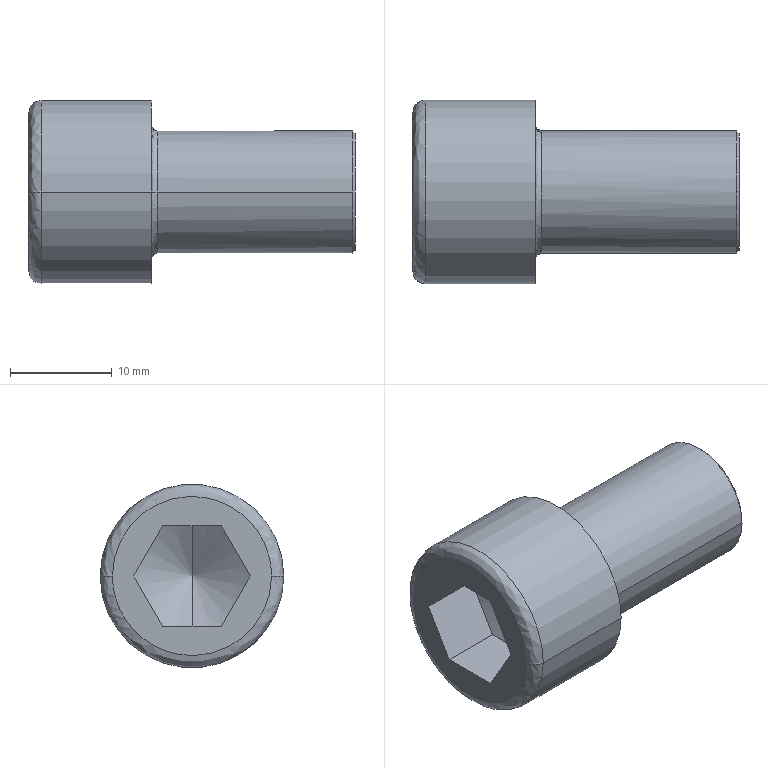Part | SolidWorks | features BaseBody 1 | 1 solid | 27 faces | box 32 x 18 x 18 mm | volume 4679 mm3 | plane 15 | spline 4 | cylinder 4 | cone 4 | commonest cylinder face diameters 12 x2 18 x2
STEP:
#1=CARTESIAN_POINT('',(0.6,6.,0.));
#2=VERTEX_POINT('',#1);
#3=CARTESIAN_POINT('',(0.6,-6.,0.));
#4=VERTEX_POINT('',#3);
#5=CARTESIAN_POINT('',(0.6,0.,0.));
#6=DIRECTION('',(1.,0.,0.));
#7=DIRECTION('',(0.,-1.,0.));
#8=AXIS2_PLACEMENT_3D('',#5,#6,#7);
#9=CIRCLE('',#8,6.);
#10=EDGE_CURVE('',#2,#4,#9,.T.);
#11=ORIENTED_EDGE('',*,*,#10,.F.);
#12=CARTESIAN_POINT('',(0.,6.6,0.));
#13=VERTEX_POINT('',#12);
#14=CARTESIAN_POINT('',(0.6,6.6,0.));
#15=DIRECTION('',(0.,0.,-1.));
#16=DIRECTION('',(0.,1.,0.));
#17=AXIS2_PLACEMENT_3D('',#14,#15,#16);
#18=CIRCLE('',#17,0.6);
#19=EDGE_CURVE('',#2,#13,#18,.T.);
#20=ORIENTED_EDGE('',*,*,#19,.T.);
#21=CARTESIAN_POINT('',(0.,-6.6,0.));
#22=VERTEX_POINT('',#21);
#23=CARTESIAN_POINT('',(0.,-6.6,0.));
#24=CARTESIAN_POINT('',(0.,-6.6,0.2019));
#25=CARTESIAN_POINT('',(0.,-6.586,0.5035));
#26=CARTESIAN_POINT('',(0.,-6.546,0.853));
#27=CARTESIAN_POINT('',(0.,-6.52,1.027));
#28=CARTESIAN_POINT('',(0.,-6.507,1.102));
#29=CARTESIAN_POINT('',(0.,-6.499,1.151));
#30=CARTESIAN_POINT('',(0.,-6.495,1.175));
#31=CARTESIAN_POINT('',(0.,-6.451,1.412));
#32=CARTESIAN_POINT('',(0.,-6.377,1.723));
#33=CARTESIAN_POINT('',(0.,-6.266,2.079));
#34=CARTESIAN_POINT('',(0.,-6.203,2.255));
#35=CARTESIAN_POINT('',(0.,-6.175,2.33));
#36=CARTESIAN_POINT('',(0.,-6.156,2.38));
#37=CARTESIAN_POINT('',(0.,-6.147,2.403));
#38=CARTESIAN_POINT('',(0.,-6.054,2.637));
#39=CARTESIAN_POINT('',(0.,-5.916,2.94));
#40=CARTESIAN_POINT('',(0.,-5.729,3.281));
#41=CARTESIAN_POINT('',(0.,-5.643,3.423));
#42=CARTESIAN_POINT('',(0.,-5.585,3.518));
#43=CARTESIAN_POINT('',(0.,-5.555,3.564));
#44=CARTESIAN_POINT('',(0.,-5.275,3.993));
#45=CARTESIAN_POINT('',(0.,-4.989,4.344));
#46=CARTESIAN_POINT('',(0.,-4.506,4.828));
#47=CARTESIAN_POINT('',(0.,-4.253,5.056));
#48=CARTESIAN_POINT('',(0.,-3.984,5.264));
#49=CARTESIAN_POINT('',(0.,-3.8,5.397));
#50=CARTESIAN_POINT('',(0.,-3.705,5.463));
#51=CARTESIAN_POINT('',(0.,-3.425,5.646));
#52=CARTESIAN_POINT('',(0.,-3.137,5.814));
#53=CARTESIAN_POINT('',(0.,-2.788,5.984));
#54=CARTESIAN_POINT('',(0.,-2.635,6.051));
#55=CARTESIAN_POINT('',(0.,-2.533,6.095));
#56=CARTESIAN_POINT('',(0.,-2.479,6.117));
#57=CARTESIAN_POINT('',(0.,-2.23,6.215));
#58=CARTESIAN_POINT('',(0.,-1.927,6.319));
#59=CARTESIAN_POINT('',(0.,-1.567,6.413));
#60=CARTESIAN_POINT('',(0.,-1.384,6.454));
#61=CARTESIAN_POINT('',(0.,-1.306,6.47));
#62=CARTESIAN_POINT('',(0.,-1.253,6.48));
#63=CARTESIAN_POINT('',(0.,-1.226,6.485));
#64=CARTESIAN_POINT('',(0.,-0.8037,6.563));
#65=CARTESIAN_POINT('',(0.,-0.404,6.6));
#66=CARTESIAN_POINT('',(0.,0.202,6.6));
#67=CARTESIAN_POINT('',(0.,0.5037,6.586));
#68=CARTESIAN_POINT('',(0.,0.8531,6.546));
#69=CARTESIAN_POINT('',(0.,1.027,6.52));
#70=CARTESIAN_POINT('',(0.,1.102,6.507));
#71=CARTESIAN_POINT('',(0.,1.151,6.499));
#72=CARTESIAN_POINT('',(0.,1.175,6.495));
#73=CARTESIAN_POINT('',(0.,1.412,6.451));
#74=CARTESIAN_POINT('',(0.,1.723,6.377));
#75=CARTESIAN_POINT('',(0.,2.079,6.266));
#76=CARTESIAN_POINT('',(0.,2.255,6.203));
#77=CARTESIAN_POINT('',(0.,2.33,6.175));
#78=CARTESIAN_POINT('',(0.,2.38,6.156));
#79=CARTESIAN_POINT('',(0.,2.403,6.147));
#80=CARTESIAN_POINT('',(0.,2.637,6.054));
#81=CARTESIAN_POINT('',(0.,2.94,5.916));
#82=CARTESIAN_POINT('',(0.,3.281,5.729));
#83=CARTESIAN_POINT('',(0.,3.423,5.643));
#84=CARTESIAN_POINT('',(0.,3.518,5.585));
#85=CARTESIAN_POINT('',(0.,3.564,5.555));
#86=CARTESIAN_POINT('',(0.,3.993,5.275));
#87=CARTESIAN_POINT('',(0.,4.344,4.989));
#88=CARTESIAN_POINT('',(0.,4.828,4.506));
#89=CARTESIAN_POINT('',(0.,5.056,4.253));
#90=CARTESIAN_POINT('',(0.,5.264,3.984));
#91=CARTESIAN_POINT('',(0.,5.397,3.8));
#92=CARTESIAN_POINT('',(0.,5.463,3.705));
#93=CARTESIAN_POINT('',(0.,5.646,3.425));
#94=CARTESIAN_POINT('',(0.,5.814,3.137));
#95=CARTESIAN_POINT('',(0.,5.984,2.788));
#96=CARTESIAN_POINT('',(0.,6.051,2.635));
#97=CARTESIAN_POINT('',(0.,6.095,2.533));
#98=CARTESIAN_POINT('',(0.,6.117,2.479));
#99=CARTESIAN_POINT('',(0.,6.215,2.23));
#100=CARTESIAN_POINT('',(0.,6.319,1.927));
#101=CARTESIAN_POINT('',(0.,6.413,1.567));
#102=CARTESIAN_POINT('',(0.,6.454,1.384));
#103=CARTESIAN_POINT('',(0.,6.47,1.306));
#104=CARTESIAN_POINT('',(0.,6.48,1.253));
#105=CARTESIAN_POINT('',(0.,6.485,1.226));
#106=CARTESIAN_POINT('',(0.,6.563,0.8038));
#107=CARTESIAN_POINT('',(0.,6.6,0.4035));
#108=CARTESIAN_POINT('',(0.,6.6,0.));
#109=B_SPLINE_CURVE_WITH_KNOTS('',3,(#23,#24,#25,#26,#27,#28,#29,#30,#31,#32,#33,#34,#35,#36,#37,#38,#39,#40,#41,#42,#43,#44,#45,#46,#47,#48,#49,#50,#51,#52,#53,#54,#55,#56,#57,#58,#59,#60,#61,#62,#63,#64,#65,#66,#67,#68,#69,#70,#71,#72,#73,#74,#75,#76,#77,#78,#79,#80,#81,#82,#83,#84,#85,#86,#87,#88,#89,#90,#91,#92,#93,#94,#95,#96,#97,#98,#99,#100,#101,#102,#103,#104,#105,#106,#107,#108),.UNSPECIFIED.,.F.,.F.,(4,1,1,1,2,2,1,1,1,2,2,1,1,2,2,2,1,2,2,1,1,2,2,1,1,1,2,2,2,1,1,1,2,2,1,1,1,2,2,1,1,2,2,2,1,2,2,1,1,2,2,1,1,1,2,2,4),(0.,0.03125,0.04688,0.05469,0.05859,0.0625,0.09375,0.1094,0.1172,0.1211,0.125,0.1563,0.1719,0.1797,0.1875,0.25,0.2813,0.2969,0.3125,0.3438,0.3594,0.3672,0.375,0.4063,0.4219,0.4297,0.4336,0.4375,0.5,0.5313,0.5469,0.5547,0.5586,0.5625,0.5938,0.6094,0.6172,0.6211,0.625,0.6563,0.6719,0.6797,0.6875,0.75,0.7813,0.7969,0.8125,0.8438,0.8594,0.8672,0.875,0.9063,0.9219,0.9297,0.9336,0.9375,1.),.UNSPECIFIED.);
#110=EDGE_CURVE('',#22,#13,#109,.T.);
#111=ORIENTED_EDGE('',*,*,#110,.F.);
#112=CARTESIAN_POINT('',(0.6,-6.6,0.));
#113=DIRECTION('',(0.,0.,1.));
#114=DIRECTION('',(0.,-1.,0.));
#115=AXIS2_PLACEMENT_3D('',#112,#113,#114);
#116=CIRCLE('',#115,0.6);
#117=EDGE_CURVE('',#4,#22,#116,.T.);
#118=ORIENTED_EDGE('',*,*,#117,.F.);
#119=EDGE_LOOP('',(#11,#20,#111,#118));
#120=FACE_OUTER_BOUND('',#119,.T.);
#121=CARTESIAN_POINT('',(0.6,-6.,0.));
#122=CARTESIAN_POINT('',(0.6,-6.,12.));
#123=CARTESIAN_POINT('',(0.6,6.,12.));
#124=CARTESIAN_POINT('',(0.6,6.,0.));
#125=CARTESIAN_POINT('',(0.2485,-6.,0.));
#126=CARTESIAN_POINT('',(0.2485,-6.,12.));
#127=CARTESIAN_POINT('',(0.2485,6.,12.));
#128=CARTESIAN_POINT('',(0.2485,6.,0.));
#129=CARTESIAN_POINT('',(0.,-6.249,0.));
#130=CARTESIAN_POINT('',(0.,-6.249,12.497));
#131=CARTESIAN_POINT('',(0.,6.249,12.497));
#132=CARTESIAN_POINT('',(0.,6.249,0.));
#133=CARTESIAN_POINT('',(0.,-6.6,0.));
#134=CARTESIAN_POINT('',(0.,-6.6,13.2));
#135=CARTESIAN_POINT('',(0.,6.6,13.2));
#136=CARTESIAN_POINT('',(0.,6.6,0.));
#137=(BOUNDED_SURFACE()B_SPLINE_SURFACE(3,3,((#121,#122,#123,#124),(#125,#126,#127,#128),(#129,#130,#131,#132),(#133,#134,#135,#136)),.UNSPECIFIED.,.F.,.F.,.T.)B_SPLINE_SURFACE_WITH_KNOTS((4,4),(4,4),(0.,1.),(0.,1.),.UNSPECIFIED.)GEOMETRIC_REPRESENTATION_ITEM()RATIONAL_B_SPLINE_SURFACE(((1.,0.3333,0.3333,1.),(0.8047,0.2682,0.2682,0.8047),(0.8047,0.2682,0.2682,0.8047),(1.,0.3333,0.3333,1.)))REPRESENTATION_ITEM('')SURFACE());
#138=ADVANCED_FACE('',(#120),#137,.F.);
#139=CARTESIAN_POINT('',(-10.8,-9.,0.));
#140=VERTEX_POINT('',#139);
#141=CARTESIAN_POINT('',(-10.8,9.,0.));
#142=VERTEX_POINT('',#141);
#143=CARTESIAN_POINT('',(-10.8,0.,0.));
#144=DIRECTION('',(1.,0.,0.));
#145=DIRECTION('',(0.,-1.,0.));
#146=AXIS2_PLACEMENT_3D('',#143,#144,#145);
#147=CIRCLE('',#146,9.);
#148=EDGE_CURVE('',#140,#142,#147,.T.);
#149=ORIENTED_EDGE('',*,*,#148,.F.);
#150=CARTESIAN_POINT('',(-12.,-7.8,0.));
#151=VERTEX_POINT('',#150);
#152=CARTESIAN_POINT('',(-10.8,-7.8,0.));
#153=DIRECTION('',(0.,0.,-1.));
#154=DIRECTION('',(0.,-1.,0.));
#155=AXIS2_PLACEMENT_3D('',#152,#153,#154);
#156=CIRCLE('',#155,1.2);
#157=EDGE_CURVE('',#140,#151,#156,.T.);
#158=ORIENTED_EDGE('',*,*,#157,.T.);
#159=CARTESIAN_POINT('',(-12.,7.8,0.));
#160=VERTEX_POINT('',#159);
#161=CARTESIAN_POINT('',(-12.,-7.8,0.));
#162=CARTESIAN_POINT('',(-12.,-7.8,-15.6));
#163=CARTESIAN_POINT('',(-12.,7.8,-15.6));
#164=CARTESIAN_POINT('',(-12.,7.8,0.));
#165=(BOUNDED_CURVE()B_SPLINE_CURVE(3,(#161,#162,#163,#164),.UNSPECIFIED.,.F.,.F.)B_SPLINE_CURVE_WITH_KNOTS((4,4),(0.,1.),.UNSPECIFIED.)CURVE()GEOMETRIC_REPRESENTATION_ITEM()RATIONAL_B_SPLINE_CURVE((1.,0.3333,0.3333,1.))REPRESENTATION_ITEM(''));
#166=EDGE_CURVE('',#151,#160,#165,.T.);
#167=ORIENTED_EDGE('',*,*,#166,.T.);
#168=CARTESIAN_POINT('',(-10.8,7.8,0.));
#169=DIRECTION('',(0.,0.,1.));
#170=DIRECTION('',(0.,1.,0.));
#171=AXIS2_PLACEMENT_3D('',#168,#169,#170);
#172=CIRCLE('',#171,1.2);
#173=EDGE_CURVE('',#142,#160,#172,.T.);
#174=ORIENTED_EDGE('',*,*,#173,.F.);
#175=EDGE_LOOP('',(#149,#158,#167,#174));
#176=FACE_OUTER_BOUND('',#175,.T.);
#177=CARTESIAN_POINT('',(-10.8,-9.,0.));
#178=CARTESIAN_POINT('',(-10.8,-9.,-18.));
#179=CARTESIAN_POINT('',(-10.8,9.,-18.));
#180=CARTESIAN_POINT('',(-10.8,9.,0.));
#181=CARTESIAN_POINT('',(-11.503,-9.,0.));
#182=CARTESIAN_POINT('',(-11.503,-9.,-18.));
#183=CARTESIAN_POINT('',(-11.503,9.,-18.));
#184=CARTESIAN_POINT('',(-11.503,9.,0.));
#185=CARTESIAN_POINT('',(-12.,-8.503,0.));
#186=CARTESIAN_POINT('',(-12.,-8.503,-17.006));
#187=CARTESIAN_POINT('',(-12.,8.503,-17.006));
#188=CARTESIAN_POINT('',(-12.,8.503,0.));
#189=CARTESIAN_POINT('',(-12.,-7.8,0.));
#190=CARTESIAN_POINT('',(-12.,-7.8,-15.6));
#191=CARTESIAN_POINT('',(-12.,7.8,-15.6));
#192=CARTESIAN_POINT('',(-12.,7.8,0.));
#193=(BOUNDED_SURFACE()B_SPLINE_SURFACE(3,3,((#177,#178,#179,#180),(#181,#182,#183,#184),(#185,#186,#187,#188),(#189,#190,#191,#192)),.UNSPECIFIED.,.F.,.F.,.T.)B_SPLINE_SURFACE_WITH_KNOTS((4,4),(4,4),(0.,1.),(0.,1.),.UNSPECIFIED.)GEOMETRIC_REPRESENTATION_ITEM()RATIONAL_B_SPLINE_SURFACE(((1.,0.3333,0.3333,1.),(0.8047,0.2682,0.2682,0.8047),(0.8047,0.2682,0.2682,0.8047),(1.,0.3333,0.3333,1.)))REPRESENTATION_ITEM('')SURFACE());
#194=ADVANCED_FACE('',(#176),#193,.T.);
#195=CARTESIAN_POINT('',(19.76,0.,6.));
#196=VERTEX_POINT('',#195);
#197=CARTESIAN_POINT('',(19.76,6.,0.));
#198=VERTEX_POINT('',#197);
#199=CARTESIAN_POINT('',(19.76,0.,0.));
#200=DIRECTION('',(-1.,0.,0.));
#201=DIRECTION('',(0.,-1.,0.));
#202=AXIS2_PLACEMENT_3D('',#199,#200,#201);
#203=CIRCLE('',#202,6.);
#204=EDGE_CURVE('',#196,#198,#203,.T.);
#205=ORIENTED_EDGE('',*,*,#204,.T.);
#206=CARTESIAN_POINT('',(20.,6.,0.));
#207=DIRECTION('',(-1.,0.,0.));
#208=VECTOR('',#207,1000.);
#209=LINE('',#206,#208);
#210=EDGE_CURVE('',#198,#2,#209,.T.);
#211=ORIENTED_EDGE('',*,*,#210,.T.);
#212=ORIENTED_EDGE('',*,*,#10,.T.);
#213=CARTESIAN_POINT('',(19.76,-6.,0.));
#214=VERTEX_POINT('',#213);
#215=CARTESIAN_POINT('',(20.,-6.,0.));
#216=DIRECTION('',(-1.,0.,0.));
#217=VECTOR('',#216,1000.);
#218=LINE('',#215,#217);
#219=EDGE_CURVE('',#214,#4,#218,.T.);
#220=ORIENTED_EDGE('',*,*,#219,.F.);
#221=CARTESIAN_POINT('',(19.76,0.,0.));
#222=DIRECTION('',(-1.,0.,0.));
#223=DIRECTION('',(0.,-1.,0.));
#224=AXIS2_PLACEMENT_3D('',#221,#222,#223);
#225=CIRCLE('',#224,6.);
#226=EDGE_CURVE('',#214,#196,#225,.T.);
#227=ORIENTED_EDGE('',*,*,#226,.T.);
#228=EDGE_LOOP('',(#205,#211,#212,#220,#227));
#229=FACE_OUTER_BOUND('',#228,.T.);
#230=CARTESIAN_POINT('',(20.,0.,0.));
#231=DIRECTION('',(-1.,0.,0.));
#232=DIRECTION('',(0.,-1.,0.));
#233=AXIS2_PLACEMENT_3D('',#230,#231,#232);
#234=CYLINDRICAL_SURFACE('',#233,6.);
#235=ADVANCED_FACE('',(#229),#234,.T.);
#236=CARTESIAN_POINT('',(20.,0.,5.76));
#237=VERTEX_POINT('',#236);
#238=CARTESIAN_POINT('',(20.,0.,-5.76));
#239=VERTEX_POINT('',#238);
#240=CARTESIAN_POINT('',(20.,0.,0.));
#241=DIRECTION('',(-1.,0.,0.));
#242=DIRECTION('',(0.,0.,1.));
#243=AXIS2_PLACEMENT_3D('',#240,#241,#242);
#244=CIRCLE('',#243,5.76);
#245=EDGE_CURVE('',#237,#239,#244,.T.);
#246=ORIENTED_EDGE('',*,*,#245,.T.);
#247=CARTESIAN_POINT('',(19.76,0.,-6.));
#248=VERTEX_POINT('',#247);
#249=CARTESIAN_POINT('',(19.76,0.,-6.));
#250=DIRECTION('',(-0.7071,0.,-0.7071));
#251=VECTOR('',#250,1000.);
#252=LINE('',#249,#251);
#253=EDGE_CURVE('',#239,#248,#252,.T.);
#254=ORIENTED_EDGE('',*,*,#253,.T.);
#255=CARTESIAN_POINT('',(19.76,0.,0.));
#256=DIRECTION('',(-1.,0.,0.));
#257=DIRECTION('',(0.,-1.,0.));
#258=AXIS2_PLACEMENT_3D('',#255,#256,#257);
#259=CIRCLE('',#258,6.);
#260=EDGE_CURVE('',#198,#248,#259,.T.);
#261=ORIENTED_EDGE('',*,*,#260,.F.);
#262=ORIENTED_EDGE('',*,*,#204,.F.);
#263=CARTESIAN_POINT('',(19.76,0.,6.));
#264=DIRECTION('',(-0.7071,0.,0.7071));
#265=VECTOR('',#264,1000.);
#266=LINE('',#263,#265);
#267=EDGE_CURVE('',#237,#196,#266,.T.);
#268=ORIENTED_EDGE('',*,*,#267,.F.);
#269=EDGE_LOOP('',(#246,#254,#261,#262,#268));
#270=FACE_OUTER_BOUND('',#269,.T.);
#271=CARTESIAN_POINT('',(19.76,0.,0.));
#272=DIRECTION('',(-1.,0.,0.));
#273=DIRECTION('',(0.,0.,1.));
#274=AXIS2_PLACEMENT_3D('',#271,#272,#273);
#275=CONICAL_SURFACE('',#274,6.,0.7854);
#276=ADVANCED_FACE('',(#270),#275,.T.);
#277=CARTESIAN_POINT('',(0.,-9.,0.));
#278=VERTEX_POINT('',#277);
#279=CARTESIAN_POINT('',(0.,9.,0.));
#280=VERTEX_POINT('',#279);
#281=CARTESIAN_POINT('',(0.,0.,0.));
#282=DIRECTION('',(-1.,0.,0.));
#283=DIRECTION('',(0.,-1.,0.));
#284=AXIS2_PLACEMENT_3D('',#281,#282,#283);
#285=CIRCLE('',#284,9.);
#286=EDGE_CURVE('',#278,#280,#285,.T.);
#287=ORIENTED_EDGE('',*,*,#286,.T.);
#288=CARTESIAN_POINT('',(-2.701,9.,0.));
#289=DIRECTION('',(-1.,0.,0.));
#290=VECTOR('',#289,1000.);
#291=LINE('',#288,#290);
#292=EDGE_CURVE('',#280,#142,#291,.T.);
#293=ORIENTED_EDGE('',*,*,#292,.T.);
#294=CARTESIAN_POINT('',(-10.8,0.,0.));
#295=DIRECTION('',(1.,0.,0.));
#296=DIRECTION('',(0.,-1.,0.));
#297=AXIS2_PLACEMENT_3D('',#294,#295,#296);
#298=CIRCLE('',#297,9.);
#299=EDGE_CURVE('',#142,#140,#298,.T.);
#300=ORIENTED_EDGE('',*,*,#299,.T.);
#301=CARTESIAN_POINT('',(-2.701,-9.,0.));
#302=DIRECTION('',(-1.,0.,0.));
#303=VECTOR('',#302,1000.);
#304=LINE('',#301,#303);
#305=EDGE_CURVE('',#278,#140,#304,.T.);
#306=ORIENTED_EDGE('',*,*,#305,.F.);
#307=EDGE_LOOP('',(#287,#293,#300,#306));
#308=FACE_OUTER_BOUND('',#307,.T.);
#309=CARTESIAN_POINT('',(-2.701,0.,0.));
#310=DIRECTION('',(-1.,0.,0.));
#311=DIRECTION('',(0.,-1.,0.));
#312=AXIS2_PLACEMENT_3D('',#309,#310,#311);
#313=CYLINDRICAL_SURFACE('',#312,9.);
#314=ADVANCED_FACE('',(#308),#313,.T.);
#315=CARTESIAN_POINT('',(-2.701,0.,0.));
#316=VERTEX_POINT('',#315);
#317=CARTESIAN_POINT('',(-6.,0.,5.715));
#318=VERTEX_POINT('',#317);
#319=CARTESIAN_POINT('',(-6.,0.,5.715));
#320=DIRECTION('',(-0.5,0.,0.866));
#321=VECTOR('',#320,1000.);
#322=LINE('',#319,#321);
#323=EDGE_CURVE('',#316,#318,#322,.T.);
#324=ORIENTED_EDGE('',*,*,#323,.F.);
#325=CARTESIAN_POINT('',(-6.,0.,-5.714));
#326=VERTEX_POINT('',#325);
#327=CARTESIAN_POINT('',(-6.,0.,-5.715));
#328=DIRECTION('',(-0.5,0.,-0.866));
#329=VECTOR('',#328,1000.);
#330=LINE('',#327,#329);
#331=EDGE_CURVE('',#316,#326,#330,.T.);
#332=ORIENTED_EDGE('',*,*,#331,.T.);
#333=CARTESIAN_POINT('',(-6.,-2.857,-4.949));
#334=VERTEX_POINT('',#333);
#335=CARTESIAN_POINT('',(-6.,0.,0.));
#336=DIRECTION('',(-1.,0.,0.));
#337=DIRECTION('',(0.,0.,1.));
#338=AXIS2_PLACEMENT_3D('',#335,#336,#337);
#339=CIRCLE('',#338,5.715);
#340=EDGE_CURVE('',#326,#334,#339,.T.);
#341=ORIENTED_EDGE('',*,*,#340,.T.);
#342=CARTESIAN_POINT('',(-6.,-5.715,0.));
#343=VERTEX_POINT('',#342);
#344=CARTESIAN_POINT('',(-6.,0.,0.));
#345=DIRECTION('',(-1.,0.,0.));
#346=DIRECTION('',(0.,0.,1.));
#347=AXIS2_PLACEMENT_3D('',#344,#345,#346);
#348=CIRCLE('',#347,5.715);
#349=EDGE_CURVE('',#334,#343,#348,.T.);
#350=ORIENTED_EDGE('',*,*,#349,.T.);
#351=CARTESIAN_POINT('',(-6.,-2.857,4.949));
#352=VERTEX_POINT('',#351);
#353=CARTESIAN_POINT('',(-6.,0.,0.));
#354=DIRECTION('',(-1.,0.,0.));
#355=DIRECTION('',(0.,0.,1.));
#356=AXIS2_PLACEMENT_3D('',#353,#354,#355);
#357=CIRCLE('',#356,5.715);
#358=EDGE_CURVE('',#343,#352,#357,.T.);
#359=ORIENTED_EDGE('',*,*,#358,.T.);
#360=CARTESIAN_POINT('',(-6.,0.,0.));
#361=DIRECTION('',(-1.,0.,0.));
#362=DIRECTION('',(0.,0.,1.));
#363=AXIS2_PLACEMENT_3D('',#360,#361,#362);
#364=CIRCLE('',#363,5.715);
#365=EDGE_CURVE('',#352,#318,#364,.T.);
#366=ORIENTED_EDGE('',*,*,#365,.T.);
#367=EDGE_LOOP('',(#324,#332,#341,#350,#359,#366));
#368=FACE_OUTER_BOUND('',#367,.T.);
#369=CARTESIAN_POINT('',(-6.,0.,0.));
#370=DIRECTION('',(-1.,0.,0.));
#371=DIRECTION('',(0.,0.,1.));
#372=AXIS2_PLACEMENT_3D('',#369,#370,#371);
#373=CONICAL_SURFACE('',#372,5.715,1.047);
#374=ADVANCED_FACE('',(#368),#373,.F.);
#375=ORIENTED_EDGE('',*,*,#210,.F.);
#376=ORIENTED_EDGE('',*,*,#260,.T.);
#377=CARTESIAN_POINT('',(19.76,0.,0.));
#378=DIRECTION('',(-1.,0.,0.));
#379=DIRECTION('',(0.,-1.,0.));
#380=AXIS2_PLACEMENT_3D('',#377,#378,#379);
#381=CIRCLE('',#380,6.);
#382=EDGE_CURVE('',#248,#214,#381,.T.);
#383=ORIENTED_EDGE('',*,*,#382,.T.);
#384=ORIENTED_EDGE('',*,*,#219,.T.);
#385=CARTESIAN_POINT('',(0.6,0.,0.));
#386=DIRECTION('',(1.,0.,0.));
#387=DIRECTION('',(0.,-1.,0.));
#388=AXIS2_PLACEMENT_3D('',#385,#386,#387);
#389=CIRCLE('',#388,6.);
#390=EDGE_CURVE('',#4,#2,#389,.T.);
#391=ORIENTED_EDGE('',*,*,#390,.T.);
#392=EDGE_LOOP('',(#375,#376,#383,#384,#391));
#393=FACE_OUTER_BOUND('',#392,.T.);
#394=CARTESIAN_POINT('',(20.,0.,0.));
#395=DIRECTION('',(-1.,0.,0.));
#396=DIRECTION('',(0.,-1.,0.));
#397=AXIS2_PLACEMENT_3D('',#394,#395,#396);
#398=CYLINDRICAL_SURFACE('',#397,6.);
#399=ADVANCED_FACE('',(#393),#398,.T.);
#400=ORIENTED_EDGE('',*,*,#19,.F.);
#401=ORIENTED_EDGE('',*,*,#390,.F.);
#402=ORIENTED_EDGE('',*,*,#117,.T.);
#403=CARTESIAN_POINT('',(0.,6.6,0.));
#404=CARTESIAN_POINT('',(0.,6.6,-0.2019));
#405=CARTESIAN_POINT('',(0.,6.586,-0.5035));
#406=CARTESIAN_POINT('',(0.,6.546,-0.853));
#407=CARTESIAN_POINT('',(0.,6.52,-1.027));
#408=CARTESIAN_POINT('',(0.,6.507,-1.102));
#409=CARTESIAN_POINT('',(0.,6.499,-1.151));
#410=CARTESIAN_POINT('',(0.,6.495,-1.175));
#411=CARTESIAN_POINT('',(0.,6.451,-1.412));
#412=CARTESIAN_POINT('',(0.,6.377,-1.723));
#413=CARTESIAN_POINT('',(0.,6.266,-2.079));
#414=CARTESIAN_POINT('',(0.,6.203,-2.255));
#415=CARTESIAN_POINT('',(0.,6.175,-2.33));
#416=CARTESIAN_POINT('',(0.,6.156,-2.38));
#417=CARTESIAN_POINT('',(0.,6.147,-2.403));
#418=CARTESIAN_POINT('',(0.,6.054,-2.637));
#419=CARTESIAN_POINT('',(0.,5.916,-2.94));
#420=CARTESIAN_POINT('',(0.,5.729,-3.281));
#421=CARTESIAN_POINT('',(0.,5.643,-3.423));
#422=CARTESIAN_POINT('',(0.,5.585,-3.518));
#423=CARTESIAN_POINT('',(0.,5.555,-3.564));
#424=CARTESIAN_POINT('',(0.,5.275,-3.993));
#425=CARTESIAN_POINT('',(0.,4.989,-4.344));
#426=CARTESIAN_POINT('',(0.,4.506,-4.828));
#427=CARTESIAN_POINT('',(0.,4.253,-5.056));
#428=CARTESIAN_POINT('',(0.,3.984,-5.264));
#429=CARTESIAN_POINT('',(0.,3.8,-5.397));
#430=CARTESIAN_POINT('',(0.,3.705,-5.463));
#431=CARTESIAN_POINT('',(0.,3.425,-5.646));
#432=CARTESIAN_POINT('',(0.,3.137,-5.814));
#433=CARTESIAN_POINT('',(0.,2.788,-5.984));
#434=CARTESIAN_POINT('',(0.,2.635,-6.051));
#435=CARTESIAN_POINT('',(0.,2.533,-6.095));
#436=CARTESIAN_POINT('',(0.,2.479,-6.117));
#437=CARTESIAN_POINT('',(0.,2.23,-6.215));
#438=CARTESIAN_POINT('',(0.,1.927,-6.319));
#439=CARTESIAN_POINT('',(0.,1.567,-6.413));
#440=CARTESIAN_POINT('',(0.,1.384,-6.454));
#441=CARTESIAN_POINT('',(0.,1.306,-6.47));
#442=CARTESIAN_POINT('',(0.,1.253,-6.48));
#443=CARTESIAN_POINT('',(0.,1.226,-6.485));
#444=CARTESIAN_POINT('',(0.,0.8037,-6.563));
#445=CARTESIAN_POINT('',(0.,0.404,-6.6));
#446=CARTESIAN_POINT('',(0.,-0.202,-6.6));
#447=CARTESIAN_POINT('',(0.,-0.5037,-6.586));
#448=CARTESIAN_POINT('',(0.,-0.8531,-6.546));
#449=CARTESIAN_POINT('',(0.,-1.027,-6.52));
#450=CARTESIAN_POINT('',(0.,-1.102,-6.507));
#451=CARTESIAN_POINT('',(0.,-1.151,-6.499));
#452=CARTESIAN_POINT('',(0.,-1.175,-6.495));
#453=CARTESIAN_POINT('',(0.,-1.412,-6.451));
#454=CARTESIAN_POINT('',(0.,-1.723,-6.377));
#455=CARTESIAN_POINT('',(0.,-2.079,-6.266));
#456=CARTESIAN_POINT('',(0.,-2.255,-6.203));
#457=CARTESIAN_POINT('',(0.,-2.33,-6.175));
#458=CARTESIAN_POINT('',(0.,-2.38,-6.156));
#459=CARTESIAN_POINT('',(0.,-2.403,-6.147));
#460=CARTESIAN_POINT('',(0.,-2.637,-6.054));
#461=CARTESIAN_POINT('',(0.,-2.94,-5.916));
#462=CARTESIAN_POINT('',(0.,-3.281,-5.729));
#463=CARTESIAN_POINT('',(0.,-3.423,-5.643));
#464=CARTESIAN_POINT('',(0.,-3.518,-5.585));
#465=CARTESIAN_POINT('',(0.,-3.564,-5.555));
#466=CARTESIAN_POINT('',(0.,-3.993,-5.275));
#467=CARTESIAN_POINT('',(0.,-4.344,-4.989));
#468=CARTESIAN_POINT('',(0.,-4.828,-4.506));
#469=CARTESIAN_POINT('',(0.,-5.056,-4.253));
#470=CARTESIAN_POINT('',(0.,-5.264,-3.984));
#471=CARTESIAN_POINT('',(0.,-5.397,-3.8));
#472=CARTESIAN_POINT('',(0.,-5.463,-3.705));
#473=CARTESIAN_POINT('',(0.,-5.646,-3.425));
#474=CARTESIAN_POINT('',(0.,-5.814,-3.137));
#475=CARTESIAN_POINT('',(0.,-5.984,-2.788));
#476=CARTESIAN_POINT('',(0.,-6.051,-2.635));
#477=CARTESIAN_POINT('',(0.,-6.095,-2.533));
#478=CARTESIAN_POINT('',(0.,-6.117,-2.479));
#479=CARTESIAN_POINT('',(0.,-6.215,-2.23));
#480=CARTESIAN_POINT('',(0.,-6.319,-1.927));
#481=CARTESIAN_POINT('',(0.,-6.413,-1.567));
#482=CARTESIAN_POINT('',(0.,-6.454,-1.384));
#483=CARTESIAN_POINT('',(0.,-6.47,-1.306));
#484=CARTESIAN_POINT('',(0.,-6.48,-1.253));
#485=CARTESIAN_POINT('',(0.,-6.485,-1.226));
#486=CARTESIAN_POINT('',(0.,-6.563,-0.8038));
#487=CARTESIAN_POINT('',(0.,-6.6,-0.4035));
#488=CARTESIAN_POINT('',(0.,-6.6,0.));
#489=B_SPLINE_CURVE_WITH_KNOTS('',3,(#403,#404,#405,#406,#407,#408,#409,#410,#411,#412,#413,#414,#415,#416,#417,#418,#419,#420,#421,#422,#423,#424,#425,#426,#427,#428,#429,#430,#431,#432,#433,#434,#435,#436,#437,#438,#439,#440,#441,#442,#443,#444,#445,#446,#447,#448,#449,#450,#451,#452,#453,#454,#455,#456,#457,#458,#459,#460,#461,#462,#463,#464,#465,#466,#467,#468,#469,#470,#471,#472,#473,#474,#475,#476,#477,#478,#479,#480,#481,#482,#483,#484,#485,#486,#487,#488),.UNSPECIFIED.,.F.,.F.,(4,1,1,1,2,2,1,1,1,2,2,1,1,2,2,2,1,2,2,1,1,2,2,1,1,1,2,2,2,1,1,1,2,2,1,1,1,2,2,1,1,2,2,2,1,2,2,1,1,2,2,1,1,1,2,2,4),(0.,0.03125,0.04688,0.05469,0.05859,0.0625,0.09375,0.1094,0.1172,0.1211,0.125,0.1563,0.1719,0.1797,0.1875,0.25,0.2813,0.2969,0.3125,0.3437,0.3594,0.3672,0.375,0.4062,0.4219,0.4297,0.4336,0.4375,0.5,0.5312,0.5469,0.5547,0.5586,0.5625,0.5937,0.6094,0.6172,0.6211,0.625,0.6562,0.6719,0.6797,0.6875,0.75,0.7812,0.7969,0.8125,0.8437,0.8594,0.8672,0.875,0.9062,0.9219,0.9297,0.9336,0.9375,1.),.UNSPECIFIED.);
#490=EDGE_CURVE('',#13,#22,#489,.T.);
#491=ORIENTED_EDGE('',*,*,#490,.F.);
#492=EDGE_LOOP('',(#400,#401,#402,#491));
#493=FACE_OUTER_BOUND('',#492,.T.);
#494=CARTESIAN_POINT('',(0.6,6.,0.));
#495=CARTESIAN_POINT('',(0.6,6.,-12.));
#496=CARTESIAN_POINT('',(0.6,-6.,-12.));
#497=CARTESIAN_POINT('',(0.6,-6.,0.));
#498=CARTESIAN_POINT('',(0.2485,6.,0.));
#499=CARTESIAN_POINT('',(0.2485,6.,-12.));
#500=CARTESIAN_POINT('',(0.2485,-6.,-12.));
#501=CARTESIAN_POINT('',(0.2485,-6.,0.));
#502=CARTESIAN_POINT('',(0.,6.249,0.));
#503=CARTESIAN_POINT('',(0.,6.249,-12.497));
#504=CARTESIAN_POINT('',(0.,-6.249,-12.497));
#505=CARTESIAN_POINT('',(0.,-6.249,0.));
#506=CARTESIAN_POINT('',(0.,6.6,0.));
#507=CARTESIAN_POINT('',(0.,6.6,-13.2));
#508=CARTESIAN_POINT('',(0.,-6.6,-13.2));
#509=CARTESIAN_POINT('',(0.,-6.6,0.));
#510=(BOUNDED_SURFACE()B_SPLINE_SURFACE(3,3,((#494,#495,#496,#497),(#498,#499,#500,#501),(#502,#503,#504,#505),(#506,#507,#508,#509)),.UNSPECIFIED.,.F.,.F.,.F.)B_SPLINE_SURFACE_WITH_KNOTS((4,4),(4,4),(0.,1.),(0.,1.),.UNSPECIFIED.)GEOMETRIC_REPRESENTATION_ITEM()RATIONAL_B_SPLINE_SURFACE(((1.,0.3333,0.3333,1.),(0.8047,0.2682,0.2682,0.8047),(0.8047,0.2682,0.2682,0.8047),(1.,0.3333,0.3333,1.)))REPRESENTATION_ITEM('')SURFACE());
#511=ADVANCED_FACE('',(#493),#510,.F.);
#512=ORIENTED_EDGE('',*,*,#253,.F.);
#513=CARTESIAN_POINT('',(20.,0.,0.));
#514=DIRECTION('',(-1.,0.,0.));
#515=DIRECTION('',(0.,0.,1.));
#516=AXIS2_PLACEMENT_3D('',#513,#514,#515);
#517=CIRCLE('',#516,5.76);
#518=EDGE_CURVE('',#239,#237,#517,.T.);
#519=ORIENTED_EDGE('',*,*,#518,.T.);
#520=ORIENTED_EDGE('',*,*,#267,.T.);
#521=ORIENTED_EDGE('',*,*,#226,.F.);
#522=ORIENTED_EDGE('',*,*,#382,.F.);
#523=EDGE_LOOP('',(#512,#519,#520,#521,#522));
#524=FACE_OUTER_BOUND('',#523,.T.);
#525=CARTESIAN_POINT('',(19.76,0.,0.));
#526=DIRECTION('',(-1.,0.,0.));
#527=DIRECTION('',(0.,0.,1.));
#528=AXIS2_PLACEMENT_3D('',#525,#526,#527);
#529=CONICAL_SURFACE('',#528,6.,0.7854);
#530=ADVANCED_FACE('',(#524),#529,.T.);
#531=ORIENTED_EDGE('',*,*,#286,.F.);
#532=CARTESIAN_POINT('',(0.,0.,0.));
#533=DIRECTION('',(-1.,0.,0.));
#534=DIRECTION('',(0.,-1.,0.));
#535=AXIS2_PLACEMENT_3D('',#532,#533,#534);
#536=CIRCLE('',#535,9.);
#537=EDGE_CURVE('',#280,#278,#536,.T.);
#538=ORIENTED_EDGE('',*,*,#537,.F.);
#539=EDGE_LOOP('',(#531,#538));
#540=FACE_OUTER_BOUND('',#539,.T.);
#541=ORIENTED_EDGE('',*,*,#490,.T.);
#542=ORIENTED_EDGE('',*,*,#110,.T.);
#543=EDGE_LOOP('',(#541,#542));
#544=FACE_BOUND('',#543,.T.);
#545=CARTESIAN_POINT('',(0.,9.,0.));
#546=DIRECTION('',(-1.,0.,0.));
#547=DIRECTION('',(0.,-1.,0.));
#548=AXIS2_PLACEMENT_3D('',#545,#546,#547);
#549=PLANE('',#548);
#550=ADVANCED_FACE('',(#540,#544),#549,.F.);
#551=ORIENTED_EDGE('',*,*,#245,.F.);
#552=ORIENTED_EDGE('',*,*,#518,.F.);
#553=EDGE_LOOP('',(#551,#552));
#554=FACE_OUTER_BOUND('',#553,.T.);
#555=CARTESIAN_POINT('',(20.,0.,0.));
#556=DIRECTION('',(1.,0.,0.));
#557=DIRECTION('',(0.,1.,0.));
#558=AXIS2_PLACEMENT_3D('',#555,#556,#557);
#559=PLANE('',#558);
#560=ADVANCED_FACE('',(#554),#559,.T.);
#561=ORIENTED_EDGE('',*,*,#292,.F.);
#562=ORIENTED_EDGE('',*,*,#537,.T.);
#563=ORIENTED_EDGE('',*,*,#305,.T.);
#564=ORIENTED_EDGE('',*,*,#148,.T.);
#565=EDGE_LOOP('',(#561,#562,#563,#564));
#566=FACE_OUTER_BOUND('',#565,.T.);
#567=CARTESIAN_POINT('',(-2.701,0.,0.));
#568=DIRECTION('',(-1.,0.,0.));
#569=DIRECTION('',(0.,-1.,0.));
#570=AXIS2_PLACEMENT_3D('',#567,#568,#569);
#571=CYLINDRICAL_SURFACE('',#570,9.);
#572=ADVANCED_FACE('',(#566),#571,.T.);
#573=ORIENTED_EDGE('',*,*,#157,.F.);
#574=ORIENTED_EDGE('',*,*,#299,.F.);
#575=ORIENTED_EDGE('',*,*,#173,.T.);
#576=CARTESIAN_POINT('',(-12.,7.8,0.));
#577=CARTESIAN_POINT('',(-12.,7.8,15.6));
#578=CARTESIAN_POINT('',(-12.,-7.8,15.6));
#579=CARTESIAN_POINT('',(-12.,-7.8,0.));
#580=(BOUNDED_CURVE()B_SPLINE_CURVE(3,(#576,#577,#578,#579),.UNSPECIFIED.,.F.,.F.)B_SPLINE_CURVE_WITH_KNOTS((4,4),(0.,1.),.UNSPECIFIED.)CURVE()GEOMETRIC_REPRESENTATION_ITEM()RATIONAL_B_SPLINE_CURVE((1.,0.3333,0.3333,1.))REPRESENTATION_ITEM(''));
#581=EDGE_CURVE('',#160,#151,#580,.T.);
#582=ORIENTED_EDGE('',*,*,#581,.T.);
#583=EDGE_LOOP('',(#573,#574,#575,#582));
#584=FACE_OUTER_BOUND('',#583,.T.);
#585=CARTESIAN_POINT('',(-10.8,9.,0.));
#586=CARTESIAN_POINT('',(-10.8,9.,18.));
#587=CARTESIAN_POINT('',(-10.8,-9.,18.));
#588=CARTESIAN_POINT('',(-10.8,-9.,0.));
#589=CARTESIAN_POINT('',(-11.503,9.,0.));
#590=CARTESIAN_POINT('',(-11.503,9.,18.));
#591=CARTESIAN_POINT('',(-11.503,-9.,18.));
#592=CARTESIAN_POINT('',(-11.503,-9.,0.));
#593=CARTESIAN_POINT('',(-12.,8.503,0.));
#594=CARTESIAN_POINT('',(-12.,8.503,17.006));
#595=CARTESIAN_POINT('',(-12.,-8.503,17.006));
#596=CARTESIAN_POINT('',(-12.,-8.503,0.));
#597=CARTESIAN_POINT('',(-12.,7.8,0.));
#598=CARTESIAN_POINT('',(-12.,7.8,15.6));
#599=CARTESIAN_POINT('',(-12.,-7.8,15.6));
#600=CARTESIAN_POINT('',(-12.,-7.8,0.));
#601=(BOUNDED_SURFACE()B_SPLINE_SURFACE(3,3,((#585,#586,#587,#588),(#589,#590,#591,#592),(#593,#594,#595,#596),(#597,#598,#599,#600)),.UNSPECIFIED.,.F.,.F.,.T.)B_SPLINE_SURFACE_WITH_KNOTS((4,4),(4,4),(0.,1.),(0.,1.),.UNSPECIFIED.)GEOMETRIC_REPRESENTATION_ITEM()RATIONAL_B_SPLINE_SURFACE(((1.,0.3333,0.3333,1.),(0.8047,0.2682,0.2682,0.8047),(0.8047,0.2682,0.2682,0.8047),(1.,0.3333,0.3333,1.)))REPRESENTATION_ITEM('')SURFACE());
#602=ADVANCED_FACE('',(#584),#601,.T.);
#603=CARTESIAN_POINT('',(-12.,2.857,-4.949));
#604=VERTEX_POINT('',#603);
#605=CARTESIAN_POINT('',(-12.,-2.857,-4.949));
#606=VERTEX_POINT('',#605);
#607=CARTESIAN_POINT('',(-12.,5.715,-4.949));
#608=DIRECTION('',(0.,-1.,0.));
#609=VECTOR('',#608,1000.);
#610=LINE('',#607,#609);
#611=EDGE_CURVE('',#604,#606,#610,.T.);
#612=ORIENTED_EDGE('',*,*,#611,.F.);
#613=CARTESIAN_POINT('',(-12.,5.715,0.));
#614=VERTEX_POINT('',#613);
#615=CARTESIAN_POINT('',(-12.,5.715,0.));
#616=DIRECTION('',(0.,-0.5,-0.866));
#617=VECTOR('',#616,1000.);
#618=LINE('',#615,#617);
#619=EDGE_CURVE('',#614,#604,#618,.T.);
#620=ORIENTED_EDGE('',*,*,#619,.F.);
#621=CARTESIAN_POINT('',(-12.,2.857,4.949));
#622=VERTEX_POINT('',#621);
#623=CARTESIAN_POINT('',(-12.,2.857,4.949));
#624=DIRECTION('',(0.,0.5,-0.866));
#625=VECTOR('',#624,1000.);
#626=LINE('',#623,#625);
#627=EDGE_CURVE('',#622,#614,#626,.T.);
#628=ORIENTED_EDGE('',*,*,#627,.F.);
#629=CARTESIAN_POINT('',(-12.,-2.857,4.949));
#630=VERTEX_POINT('',#629);
#631=CARTESIAN_POINT('',(-12.,5.715,4.949));
#632=DIRECTION('',(0.,1.,0.));
#633=VECTOR('',#632,1000.);
#634=LINE('',#631,#633);
#635=EDGE_CURVE('',#630,#622,#634,.T.);
#636=ORIENTED_EDGE('',*,*,#635,.F.);
#637=CARTESIAN_POINT('',(-12.,-5.715,0.));
#638=VERTEX_POINT('',#637);
#639=CARTESIAN_POINT('',(-12.,-5.715,0.));
#640=DIRECTION('',(0.,0.5,0.866));
#641=VECTOR('',#640,1000.);
#642=LINE('',#639,#641);
#643=EDGE_CURVE('',#638,#630,#642,.T.);
#644=ORIENTED_EDGE('',*,*,#643,.F.);
#645=CARTESIAN_POINT('',(-12.,-2.857,-4.949));
#646=DIRECTION('',(0.,-0.5,0.866));
#647=VECTOR('',#646,1000.);
#648=LINE('',#645,#647);
#649=EDGE_CURVE('',#606,#638,#648,.T.);
#650=ORIENTED_EDGE('',*,*,#649,.F.);
#651=EDGE_LOOP('',(#612,#620,#628,#636,#644,#650));
#652=FACE_BOUND('',#651,.T.);
#653=ORIENTED_EDGE('',*,*,#581,.F.);
#654=ORIENTED_EDGE('',*,*,#166,.F.);
#655=EDGE_LOOP('',(#653,#654));
#656=FACE_OUTER_BOUND('',#655,.T.);
#657=CARTESIAN_POINT('',(-12.,5.715,0.));
#658=DIRECTION('',(1.,0.,0.));
#659=DIRECTION('',(0.,1.,0.));
#660=AXIS2_PLACEMENT_3D('',#657,#658,#659);
#661=PLANE('',#660);
#662=ADVANCED_FACE('',(#652,#656),#661,.F.);
#663=CARTESIAN_POINT('',(-6.,-2.857,-4.949));
#664=DIRECTION('',(0.,-0.5,0.866));
#665=VECTOR('',#664,1000.);
#666=LINE('',#663,#665);
#667=EDGE_CURVE('',#334,#343,#666,.T.);
#668=ORIENTED_EDGE('',*,*,#667,.F.);
#669=CARTESIAN_POINT('',(-6.,-2.857,-4.949));
#670=DIRECTION('',(1.,0.,0.));
#671=VECTOR('',#670,1000.);
#672=LINE('',#669,#671);
#673=EDGE_CURVE('',#606,#334,#672,.T.);
#674=ORIENTED_EDGE('',*,*,#673,.F.);
#675=ORIENTED_EDGE('',*,*,#649,.T.);
#676=CARTESIAN_POINT('',(-6.,-5.715,0.));
#677=DIRECTION('',(-1.,0.,0.));
#678=VECTOR('',#677,1000.);
#679=LINE('',#676,#678);
#680=EDGE_CURVE('',#343,#638,#679,.T.);
#681=ORIENTED_EDGE('',*,*,#680,.F.);
#682=EDGE_LOOP('',(#668,#674,#675,#681));
#683=FACE_OUTER_BOUND('',#682,.T.);
#684=CARTESIAN_POINT('',(-6.,-2.857,-4.949));
#685=DIRECTION('',(0.,-0.866,-0.5));
#686=DIRECTION('',(0.,0.5,-0.866));
#687=AXIS2_PLACEMENT_3D('',#684,#685,#686);
#688=PLANE('',#687);
#689=ADVANCED_FACE('',(#683),#688,.F.);
#690=CARTESIAN_POINT('',(-6.,2.857,-4.949));
#691=VERTEX_POINT('',#690);
#692=CARTESIAN_POINT('',(-6.,2.857,-4.949));
#693=DIRECTION('',(0.,-1.,0.));
#694=VECTOR('',#693,1000.);
#695=LINE('',#692,#694);
#696=EDGE_CURVE('',#691,#334,#695,.T.);
#697=ORIENTED_EDGE('',*,*,#696,.F.);
#698=CARTESIAN_POINT('',(-6.,2.857,-4.949));
#699=DIRECTION('',(1.,0.,0.));
#700=VECTOR('',#699,1000.);
#701=LINE('',#698,#700);
#702=EDGE_CURVE('',#604,#691,#701,.T.);
#703=ORIENTED_EDGE('',*,*,#702,.F.);
#704=ORIENTED_EDGE('',*,*,#611,.T.);
#705=ORIENTED_EDGE('',*,*,#673,.T.);
#706=EDGE_LOOP('',(#697,#703,#704,#705));
#707=FACE_OUTER_BOUND('',#706,.T.);
#708=CARTESIAN_POINT('',(-6.,2.857,-4.949));
#709=DIRECTION('',(0.,0.,-1.));
#710=DIRECTION('',(0.,1.,0.));
#711=AXIS2_PLACEMENT_3D('',#708,#709,#710);
#712=PLANE('',#711);
#713=ADVANCED_FACE('',(#707),#712,.F.);
#714=CARTESIAN_POINT('',(-6.,5.715,0.));
#715=VERTEX_POINT('',#714);
#716=CARTESIAN_POINT('',(-6.,5.715,0.));
#717=DIRECTION('',(0.,-0.5,-0.866));
#718=VECTOR('',#717,1000.);
#719=LINE('',#716,#718);
#720=EDGE_CURVE('',#715,#691,#719,.T.);
#721=ORIENTED_EDGE('',*,*,#720,.F.);
#722=CARTESIAN_POINT('',(-6.,5.715,0.));
#723=DIRECTION('',(1.,0.,0.));
#724=VECTOR('',#723,1000.);
#725=LINE('',#722,#724);
#726=EDGE_CURVE('',#614,#715,#725,.T.);
#727=ORIENTED_EDGE('',*,*,#726,.F.);
#728=ORIENTED_EDGE('',*,*,#619,.T.);
#729=ORIENTED_EDGE('',*,*,#702,.T.);
#730=EDGE_LOOP('',(#721,#727,#728,#729));
#731=FACE_OUTER_BOUND('',#730,.T.);
#732=CARTESIAN_POINT('',(-6.,5.715,0.));
#733=DIRECTION('',(0.,0.866,-0.5));
#734=DIRECTION('',(0.,0.5,0.866));
#735=AXIS2_PLACEMENT_3D('',#732,#733,#734);
#736=PLANE('',#735);
#737=ADVANCED_FACE('',(#731),#736,.F.);
#738=CARTESIAN_POINT('',(-6.,2.857,4.949));
#739=VERTEX_POINT('',#738);
#740=CARTESIAN_POINT('',(-6.,2.857,4.949));
#741=DIRECTION('',(0.,0.5,-0.866));
#742=VECTOR('',#741,1000.);
#743=LINE('',#740,#742);
#744=EDGE_CURVE('',#739,#715,#743,.T.);
#745=ORIENTED_EDGE('',*,*,#744,.F.);
#746=CARTESIAN_POINT('',(-6.,2.857,4.949));
#747=DIRECTION('',(1.,0.,0.));
#748=VECTOR('',#747,1000.);
#749=LINE('',#746,#748);
#750=EDGE_CURVE('',#622,#739,#749,.T.);
#751=ORIENTED_EDGE('',*,*,#750,.F.);
#752=ORIENTED_EDGE('',*,*,#627,.T.);
#753=ORIENTED_EDGE('',*,*,#726,.T.);
#754=EDGE_LOOP('',(#745,#751,#752,#753));
#755=FACE_OUTER_BOUND('',#754,.T.);
#756=CARTESIAN_POINT('',(-6.,2.857,4.949));
#757=DIRECTION('',(0.,0.866,0.5));
#758=DIRECTION('',(0.,-0.5,0.866));
#759=AXIS2_PLACEMENT_3D('',#756,#757,#758);
#760=PLANE('',#759);
#761=ADVANCED_FACE('',(#755),#760,.F.);
#762=CARTESIAN_POINT('',(-6.,-2.857,4.949));
#763=DIRECTION('',(0.,1.,0.));
#764=VECTOR('',#763,1000.);
#765=LINE('',#762,#764);
#766=EDGE_CURVE('',#352,#739,#765,.T.);
#767=ORIENTED_EDGE('',*,*,#766,.F.);
#768=CARTESIAN_POINT('',(-6.,-2.857,4.949));
#769=DIRECTION('',(1.,0.,0.));
#770=VECTOR('',#769,1000.);
#771=LINE('',#768,#770);
#772=EDGE_CURVE('',#630,#352,#771,.T.);
#773=ORIENTED_EDGE('',*,*,#772,.F.);
#774=ORIENTED_EDGE('',*,*,#635,.T.);
#775=ORIENTED_EDGE('',*,*,#750,.T.);
#776=EDGE_LOOP('',(#767,#773,#774,#775));
#777=FACE_OUTER_BOUND('',#776,.T.);
#778=CARTESIAN_POINT('',(-6.,-2.857,4.949));
#779=DIRECTION('',(0.,0.,1.));
#780=DIRECTION('',(1.,0.,0.));
#781=AXIS2_PLACEMENT_3D('',#778,#779,#780);
#782=PLANE('',#781);
#783=ADVANCED_FACE('',(#777),#782,.F.);
#784=CARTESIAN_POINT('',(-6.,-5.714,0.));
#785=DIRECTION('',(0.,0.5,0.866));
#786=VECTOR('',#785,1000.);
#787=LINE('',#784,#786);
#788=EDGE_CURVE('',#343,#352,#787,.T.);
#789=ORIENTED_EDGE('',*,*,#788,.F.);
#790=ORIENTED_EDGE('',*,*,#680,.T.);
#791=ORIENTED_EDGE('',*,*,#643,.T.);
#792=ORIENTED_EDGE('',*,*,#772,.T.);
#793=EDGE_LOOP('',(#789,#790,#791,#792));
#794=FACE_OUTER_BOUND('',#793,.T.);
#795=CARTESIAN_POINT('',(-6.,-5.714,0.));
#796=DIRECTION('',(0.,-0.866,0.5));
#797=DIRECTION('',(0.,-0.5,-0.866));
#798=AXIS2_PLACEMENT_3D('',#795,#796,#797);
#799=PLANE('',#798);
#800=ADVANCED_FACE('',(#794),#799,.F.);
#801=ORIENTED_EDGE('',*,*,#667,.T.);
#802=ORIENTED_EDGE('',*,*,#349,.F.);
#803=EDGE_LOOP('',(#801,#802));
#804=FACE_OUTER_BOUND('',#803,.T.);
#805=CARTESIAN_POINT('',(-6.,0.,0.));
#806=DIRECTION('',(-1.,0.,0.));
#807=DIRECTION('',(0.,-1.,0.));
#808=AXIS2_PLACEMENT_3D('',#805,#806,#807);
#809=PLANE('',#808);
#810=ADVANCED_FACE('',(#804),#809,.F.);
#811=ORIENTED_EDGE('',*,*,#696,.T.);
#812=ORIENTED_EDGE('',*,*,#340,.F.);
#813=CARTESIAN_POINT('',(-6.,0.,0.));
#814=DIRECTION('',(-1.,0.,0.));
#815=DIRECTION('',(0.,0.,1.));
#816=AXIS2_PLACEMENT_3D('',#813,#814,#815);
#817=CIRCLE('',#816,5.715);
#818=EDGE_CURVE('',#691,#326,#817,.T.);
#819=ORIENTED_EDGE('',*,*,#818,.F.);
#820=EDGE_LOOP('',(#811,#812,#819));
#821=FACE_OUTER_BOUND('',#820,.T.);
#822=CARTESIAN_POINT('',(-6.,0.,0.));
#823=DIRECTION('',(-1.,0.,0.));
#824=DIRECTION('',(0.,-1.,0.));
#825=AXIS2_PLACEMENT_3D('',#822,#823,#824);
#826=PLANE('',#825);
#827=ADVANCED_FACE('',(#821),#826,.F.);
#828=ORIENTED_EDGE('',*,*,#720,.T.);
#829=CARTESIAN_POINT('',(-6.,0.,0.));
#830=DIRECTION('',(-1.,0.,0.));
#831=DIRECTION('',(0.,0.,1.));
#832=AXIS2_PLACEMENT_3D('',#829,#830,#831);
#833=CIRCLE('',#832,5.715);
#834=EDGE_CURVE('',#715,#691,#833,.T.);
#835=ORIENTED_EDGE('',*,*,#834,.F.);
#836=EDGE_LOOP('',(#828,#835));
#837=FACE_OUTER_BOUND('',#836,.T.);
#838=CARTESIAN_POINT('',(-6.,0.,0.));
#839=DIRECTION('',(-1.,0.,0.));
#840=DIRECTION('',(0.,-1.,0.));
#841=AXIS2_PLACEMENT_3D('',#838,#839,#840);
#842=PLANE('',#841);
#843=ADVANCED_FACE('',(#837),#842,.F.);
#844=ORIENTED_EDGE('',*,*,#744,.T.);
#845=CARTESIAN_POINT('',(-6.,0.,0.));
#846=DIRECTION('',(-1.,0.,0.));
#847=DIRECTION('',(0.,0.,1.));
#848=AXIS2_PLACEMENT_3D('',#845,#846,#847);
#849=CIRCLE('',#848,5.715);
#850=EDGE_CURVE('',#739,#715,#849,.T.);
#851=ORIENTED_EDGE('',*,*,#850,.F.);
#852=EDGE_LOOP('',(#844,#851));
#853=FACE_OUTER_BOUND('',#852,.T.);
#854=CARTESIAN_POINT('',(-6.,0.,0.));
#855=DIRECTION('',(-1.,0.,0.));
#856=DIRECTION('',(0.,-1.,0.));
#857=AXIS2_PLACEMENT_3D('',#854,#855,#856);
#858=PLANE('',#857);
#859=ADVANCED_FACE('',(#853),#858,.F.);
#860=ORIENTED_EDGE('',*,*,#766,.T.);
#861=CARTESIAN_POINT('',(-6.,0.,0.));
#862=DIRECTION('',(-1.,0.,0.));
#863=DIRECTION('',(0.,0.,1.));
#864=AXIS2_PLACEMENT_3D('',#861,#862,#863);
#865=CIRCLE('',#864,5.715);
#866=EDGE_CURVE('',#318,#739,#865,.T.);
#867=ORIENTED_EDGE('',*,*,#866,.F.);
#868=ORIENTED_EDGE('',*,*,#365,.F.);
#869=EDGE_LOOP('',(#860,#867,#868));
#870=FACE_OUTER_BOUND('',#869,.T.);
#871=CARTESIAN_POINT('',(-6.,0.,0.));
#872=DIRECTION('',(-1.,0.,0.));
#873=DIRECTION('',(0.,-1.,0.));
#874=AXIS2_PLACEMENT_3D('',#871,#872,#873);
#875=PLANE('',#874);
#876=ADVANCED_FACE('',(#870),#875,.F.);
#877=ORIENTED_EDGE('',*,*,#788,.T.);
#878=ORIENTED_EDGE('',*,*,#358,.F.);
#879=EDGE_LOOP('',(#877,#878));
#880=FACE_OUTER_BOUND('',#879,.T.);
#881=CARTESIAN_POINT('',(-6.,0.,0.));
#882=DIRECTION('',(-1.,0.,0.));
#883=DIRECTION('',(0.,-1.,0.));
#884=AXIS2_PLACEMENT_3D('',#881,#882,#883);
#885=PLANE('',#884);
#886=ADVANCED_FACE('',(#880),#885,.F.);
#887=ORIENTED_EDGE('',*,*,#331,.F.);
#888=ORIENTED_EDGE('',*,*,#323,.T.);
#889=ORIENTED_EDGE('',*,*,#866,.T.);
#890=ORIENTED_EDGE('',*,*,#850,.T.);
#891=ORIENTED_EDGE('',*,*,#834,.T.);
#892=ORIENTED_EDGE('',*,*,#818,.T.);
#893=EDGE_LOOP('',(#887,#888,#889,#890,#891,#892));
#894=FACE_OUTER_BOUND('',#893,.T.);
#895=CARTESIAN_POINT('',(-6.,0.,0.));
#896=DIRECTION('',(-1.,0.,0.));
#897=DIRECTION('',(0.,0.,1.));
#898=AXIS2_PLACEMENT_3D('',#895,#896,#897);
#899=CONICAL_SURFACE('',#898,5.715,1.047);
#900=ADVANCED_FACE('',(#894),#899,.F.);
#901=CLOSED_SHELL('',(#138,#194,#235,#276,#314,#374,#399,#511,#530,#550,#560,#572,#602,#662,#689,#713,#737,#761,#783,#800,#810,#827,#843,#859,#876,#886,#900));
#902=MANIFOLD_SOLID_BREP('',#901);
#903=CARTESIAN_POINT('',(0.,0.,0.));
#904=DIRECTION('',(0.,0.,1.));
#905=DIRECTION('',(1.,0.,0.));
#906=AXIS2_PLACEMENT_3D('',#903,#904,#905);
#907=(LENGTH_UNIT()NAMED_UNIT(*)SI_UNIT(.MILLI.,.METRE.));
#908=UNCERTAINTY_MEASURE_WITH_UNIT(LENGTH_MEASURE(0.00001),#907,'','');
#909=(NAMED_UNIT(*)PLANE_ANGLE_UNIT()SI_UNIT($,.RADIAN.));
#910=(NAMED_UNIT(*)SI_UNIT($,.STERADIAN.)SOLID_ANGLE_UNIT());
#911=(GEOMETRIC_REPRESENTATION_CONTEXT(3)GLOBAL_UNCERTAINTY_ASSIGNED_CONTEXT((#908))GLOBAL_UNIT_ASSIGNED_CONTEXT((#907,#909,#910))REPRESENTATION_CONTEXT('',''));
#912=ADVANCED_BREP_SHAPE_REPRESENTATION('',(#902,#906),#911);